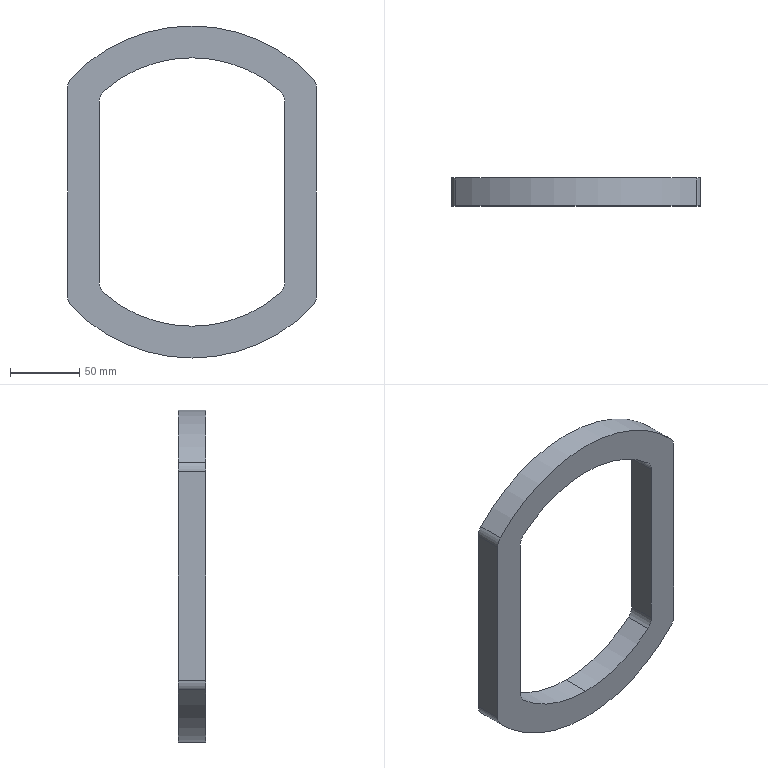Part | SolidWorks | features Extrusion 1, Fillet 1 | 1 solid | 20 faces | box 180 x 20 x 240 mm | volume 299340 mm3 | cylinder 14 | plane 6 | commonest cylinder face diameters 20 x8 194 x3 240 x3
STEP:
#1=CARTESIAN_POINT('',(63.552,20.,-73.282));
#2=VERTEX_POINT('',#1);
#3=CARTESIAN_POINT('',(0.,20.,-97.));
#4=VERTEX_POINT('',#3);
#5=CARTESIAN_POINT('',(0.,20.,0.));
#6=DIRECTION('',(0.,1.,0.));
#7=DIRECTION('',(0.,0.,1.));
#8=AXIS2_PLACEMENT_3D('',#5,#6,#7);
#9=CIRCLE('',#8,97.);
#10=EDGE_CURVE('',#2,#4,#9,.T.);
#11=ORIENTED_EDGE('',*,*,#10,.T.);
#12=CARTESIAN_POINT('',(0.,0.,-97.));
#13=VERTEX_POINT('',#12);
#14=CARTESIAN_POINT('',(0.,20.,-97.));
#15=DIRECTION('',(0.,-1.,0.));
#16=VECTOR('',#15,1000.);
#17=LINE('',#14,#16);
#18=EDGE_CURVE('',#4,#13,#17,.T.);
#19=ORIENTED_EDGE('',*,*,#18,.T.);
#20=CARTESIAN_POINT('',(63.552,0.,-73.282));
#21=VERTEX_POINT('',#20);
#22=CARTESIAN_POINT('',(0.,0.,0.));
#23=DIRECTION('',(0.,1.,0.));
#24=DIRECTION('',(0.,0.,1.));
#25=AXIS2_PLACEMENT_3D('',#22,#23,#24);
#26=CIRCLE('',#25,97.);
#27=EDGE_CURVE('',#21,#13,#26,.T.);
#28=ORIENTED_EDGE('',*,*,#27,.F.);
#29=CARTESIAN_POINT('',(63.552,20.,-73.282));
#30=DIRECTION('',(0.,1.,0.));
#31=VECTOR('',#30,1000.);
#32=LINE('',#29,#31);
#33=EDGE_CURVE('',#21,#2,#32,.T.);
#34=ORIENTED_EDGE('',*,*,#33,.T.);
#35=EDGE_LOOP('',(#11,#19,#28,#34));
#36=FACE_OUTER_BOUND('',#35,.T.);
#37=CARTESIAN_POINT('',(0.,20.,0.));
#38=DIRECTION('',(0.,-1.,0.));
#39=DIRECTION('',(0.,0.,-1.));
#40=AXIS2_PLACEMENT_3D('',#37,#38,#39);
#41=CYLINDRICAL_SURFACE('',#40,97.);
#42=ADVANCED_FACE('',(#36),#41,.F.);
#43=CARTESIAN_POINT('',(0.,20.,-120.));
#44=VERTEX_POINT('',#43);
#45=CARTESIAN_POINT('',(-87.273,20.,-82.362));
#46=VERTEX_POINT('',#45);
#47=CARTESIAN_POINT('',(0.,20.,0.));
#48=DIRECTION('',(0.,1.,0.));
#49=DIRECTION('',(0.,0.,1.));
#50=AXIS2_PLACEMENT_3D('',#47,#48,#49);
#51=CIRCLE('',#50,120.);
#52=EDGE_CURVE('',#44,#46,#51,.T.);
#53=ORIENTED_EDGE('',*,*,#52,.F.);
#54=CARTESIAN_POINT('',(0.,0.,-120.));
#55=VERTEX_POINT('',#54);
#56=CARTESIAN_POINT('',(0.,20.,-120.));
#57=DIRECTION('',(0.,-1.,0.));
#58=VECTOR('',#57,1000.);
#59=LINE('',#56,#58);
#60=EDGE_CURVE('',#44,#55,#59,.T.);
#61=ORIENTED_EDGE('',*,*,#60,.T.);
#62=CARTESIAN_POINT('',(-87.273,0.,-82.362));
#63=VERTEX_POINT('',#62);
#64=CARTESIAN_POINT('',(0.,0.,0.));
#65=DIRECTION('',(0.,1.,0.));
#66=DIRECTION('',(0.,0.,1.));
#67=AXIS2_PLACEMENT_3D('',#64,#65,#66);
#68=CIRCLE('',#67,120.);
#69=EDGE_CURVE('',#55,#63,#68,.T.);
#70=ORIENTED_EDGE('',*,*,#69,.T.);
#71=CARTESIAN_POINT('',(-87.273,20.,-82.362));
#72=DIRECTION('',(0.,-1.,0.));
#73=VECTOR('',#72,1000.);
#74=LINE('',#71,#73);
#75=EDGE_CURVE('',#46,#63,#74,.T.);
#76=ORIENTED_EDGE('',*,*,#75,.F.);
#77=EDGE_LOOP('',(#53,#61,#70,#76));
#78=FACE_OUTER_BOUND('',#77,.T.);
#79=CARTESIAN_POINT('',(0.,20.,0.));
#80=DIRECTION('',(0.,-1.,0.));
#81=DIRECTION('',(0.,0.,-1.));
#82=AXIS2_PLACEMENT_3D('',#79,#80,#81);
#83=CYLINDRICAL_SURFACE('',#82,120.);
#84=ADVANCED_FACE('',(#78),#83,.T.);
#85=CARTESIAN_POINT('',(90.,20.,-75.498));
#86=VERTEX_POINT('',#85);
#87=CARTESIAN_POINT('',(87.273,20.,-82.362));
#88=VERTEX_POINT('',#87);
#89=CARTESIAN_POINT('',(80.,20.,-75.498));
#90=DIRECTION('',(0.,1.,0.));
#91=DIRECTION('',(0.,0.,1.));
#92=AXIS2_PLACEMENT_3D('',#89,#90,#91);
#93=CIRCLE('',#92,10.);
#94=EDGE_CURVE('',#86,#88,#93,.T.);
#95=ORIENTED_EDGE('',*,*,#94,.T.);
#96=CARTESIAN_POINT('',(0.,20.,0.));
#97=DIRECTION('',(0.,1.,0.));
#98=DIRECTION('',(0.,0.,1.));
#99=AXIS2_PLACEMENT_3D('',#96,#97,#98);
#100=CIRCLE('',#99,120.);
#101=EDGE_CURVE('',#88,#44,#100,.T.);
#102=ORIENTED_EDGE('',*,*,#101,.T.);
#103=ORIENTED_EDGE('',*,*,#52,.T.);
#104=CARTESIAN_POINT('',(-90.,20.,-75.498));
#105=VERTEX_POINT('',#104);
#106=CARTESIAN_POINT('',(-80.,20.,-75.498));
#107=DIRECTION('',(0.,1.,0.));
#108=DIRECTION('',(0.,0.,1.));
#109=AXIS2_PLACEMENT_3D('',#106,#107,#108);
#110=CIRCLE('',#109,10.);
#111=EDGE_CURVE('',#46,#105,#110,.T.);
#112=ORIENTED_EDGE('',*,*,#111,.T.);
#113=CARTESIAN_POINT('',(-90.,20.,75.498));
#114=VERTEX_POINT('',#113);
#115=CARTESIAN_POINT('',(-90.,20.,-75.498));
#116=DIRECTION('',(0.,0.,1.));
#117=VECTOR('',#116,1000.);
#118=LINE('',#115,#117);
#119=EDGE_CURVE('',#105,#114,#118,.T.);
#120=ORIENTED_EDGE('',*,*,#119,.T.);
#121=CARTESIAN_POINT('',(-87.273,20.,82.362));
#122=VERTEX_POINT('',#121);
#123=CARTESIAN_POINT('',(-80.,20.,75.498));
#124=DIRECTION('',(0.,1.,0.));
#125=DIRECTION('',(0.,0.,1.));
#126=AXIS2_PLACEMENT_3D('',#123,#124,#125);
#127=CIRCLE('',#126,10.);
#128=EDGE_CURVE('',#114,#122,#127,.T.);
#129=ORIENTED_EDGE('',*,*,#128,.T.);
#130=CARTESIAN_POINT('',(87.273,20.,82.362));
#131=VERTEX_POINT('',#130);
#132=CARTESIAN_POINT('',(0.,20.,0.));
#133=DIRECTION('',(0.,1.,0.));
#134=DIRECTION('',(0.,0.,1.));
#135=AXIS2_PLACEMENT_3D('',#132,#133,#134);
#136=CIRCLE('',#135,120.);
#137=EDGE_CURVE('',#122,#131,#136,.T.);
#138=ORIENTED_EDGE('',*,*,#137,.T.);
#139=CARTESIAN_POINT('',(90.,20.,75.498));
#140=VERTEX_POINT('',#139);
#141=CARTESIAN_POINT('',(80.,20.,75.498));
#142=DIRECTION('',(0.,1.,0.));
#143=DIRECTION('',(0.,0.,1.));
#144=AXIS2_PLACEMENT_3D('',#141,#142,#143);
#145=CIRCLE('',#144,10.);
#146=EDGE_CURVE('',#131,#140,#145,.T.);
#147=ORIENTED_EDGE('',*,*,#146,.T.);
#148=CARTESIAN_POINT('',(90.,20.,75.498));
#149=DIRECTION('',(0.,0.,-1.));
#150=VECTOR('',#149,1000.);
#151=LINE('',#148,#150);
#152=EDGE_CURVE('',#140,#86,#151,.T.);
#153=ORIENTED_EDGE('',*,*,#152,.T.);
#154=EDGE_LOOP('',(#95,#102,#103,#112,#120,#129,#138,#147,#153));
#155=FACE_OUTER_BOUND('',#154,.T.);
#156=CARTESIAN_POINT('',(67.,20.,65.727));
#157=VERTEX_POINT('',#156);
#158=CARTESIAN_POINT('',(67.,20.,-65.727));
#159=VERTEX_POINT('',#158);
#160=CARTESIAN_POINT('',(67.,20.,70.143));
#161=DIRECTION('',(0.,0.,-1.));
#162=VECTOR('',#161,1000.);
#163=LINE('',#160,#162);
#164=EDGE_CURVE('',#157,#159,#163,.T.);
#165=ORIENTED_EDGE('',*,*,#164,.F.);
#166=CARTESIAN_POINT('',(63.552,20.,73.282));
#167=VERTEX_POINT('',#166);
#168=CARTESIAN_POINT('',(57.,20.,65.727));
#169=DIRECTION('',(0.,-1.,0.));
#170=DIRECTION('',(0.,0.,1.));
#171=AXIS2_PLACEMENT_3D('',#168,#169,#170);
#172=CIRCLE('',#171,10.);
#173=EDGE_CURVE('',#157,#167,#172,.T.);
#174=ORIENTED_EDGE('',*,*,#173,.T.);
#175=CARTESIAN_POINT('',(-63.552,20.,73.282));
#176=VERTEX_POINT('',#175);
#177=CARTESIAN_POINT('',(0.,20.,0.));
#178=DIRECTION('',(0.,1.,0.));
#179=DIRECTION('',(0.,0.,1.));
#180=AXIS2_PLACEMENT_3D('',#177,#178,#179);
#181=CIRCLE('',#180,97.);
#182=EDGE_CURVE('',#176,#167,#181,.T.);
#183=ORIENTED_EDGE('',*,*,#182,.F.);
#184=CARTESIAN_POINT('',(-67.,20.,65.727));
#185=VERTEX_POINT('',#184);
#186=CARTESIAN_POINT('',(-57.,20.,65.727));
#187=DIRECTION('',(0.,-1.,0.));
#188=DIRECTION('',(0.,0.,1.));
#189=AXIS2_PLACEMENT_3D('',#186,#187,#188);
#190=CIRCLE('',#189,10.);
#191=EDGE_CURVE('',#176,#185,#190,.T.);
#192=ORIENTED_EDGE('',*,*,#191,.T.);
#193=CARTESIAN_POINT('',(-67.,20.,-65.727));
#194=VERTEX_POINT('',#193);
#195=CARTESIAN_POINT('',(-67.,20.,-70.143));
#196=DIRECTION('',(0.,0.,1.));
#197=VECTOR('',#196,1000.);
#198=LINE('',#195,#197);
#199=EDGE_CURVE('',#194,#185,#198,.T.);
#200=ORIENTED_EDGE('',*,*,#199,.F.);
#201=CARTESIAN_POINT('',(-63.552,20.,-73.282));
#202=VERTEX_POINT('',#201);
#203=CARTESIAN_POINT('',(-57.,20.,-65.727));
#204=DIRECTION('',(0.,-1.,0.));
#205=DIRECTION('',(0.,0.,1.));
#206=AXIS2_PLACEMENT_3D('',#203,#204,#205);
#207=CIRCLE('',#206,10.);
#208=EDGE_CURVE('',#194,#202,#207,.T.);
#209=ORIENTED_EDGE('',*,*,#208,.T.);
#210=CARTESIAN_POINT('',(0.,20.,0.));
#211=DIRECTION('',(0.,1.,0.));
#212=DIRECTION('',(0.,0.,1.));
#213=AXIS2_PLACEMENT_3D('',#210,#211,#212);
#214=CIRCLE('',#213,97.);
#215=EDGE_CURVE('',#4,#202,#214,.T.);
#216=ORIENTED_EDGE('',*,*,#215,.F.);
#217=ORIENTED_EDGE('',*,*,#10,.F.);
#218=CARTESIAN_POINT('',(57.,20.,-65.727));
#219=DIRECTION('',(0.,-1.,0.));
#220=DIRECTION('',(0.,0.,1.));
#221=AXIS2_PLACEMENT_3D('',#218,#219,#220);
#222=CIRCLE('',#221,10.);
#223=EDGE_CURVE('',#2,#159,#222,.T.);
#224=ORIENTED_EDGE('',*,*,#223,.T.);
#225=EDGE_LOOP('',(#165,#174,#183,#192,#200,#209,#216,#217,#224));
#226=FACE_BOUND('',#225,.T.);
#227=CARTESIAN_POINT('',(80.,20.,-75.498));
#228=DIRECTION('',(0.,1.,0.));
#229=DIRECTION('',(0.,0.,1.));
#230=AXIS2_PLACEMENT_3D('',#227,#228,#229);
#231=PLANE('',#230);
#232=ADVANCED_FACE('',(#155,#226),#231,.T.);
#233=CARTESIAN_POINT('',(90.,0.,-75.498));
#234=VERTEX_POINT('',#233);
#235=CARTESIAN_POINT('',(87.273,0.,-82.362));
#236=VERTEX_POINT('',#235);
#237=CARTESIAN_POINT('',(80.,0.,-75.498));
#238=DIRECTION('',(0.,1.,0.));
#239=DIRECTION('',(0.,0.,1.));
#240=AXIS2_PLACEMENT_3D('',#237,#238,#239);
#241=CIRCLE('',#240,10.);
#242=EDGE_CURVE('',#234,#236,#241,.T.);
#243=ORIENTED_EDGE('',*,*,#242,.F.);
#244=CARTESIAN_POINT('',(90.,0.,75.498));
#245=VERTEX_POINT('',#244);
#246=CARTESIAN_POINT('',(90.,0.,75.498));
#247=DIRECTION('',(0.,0.,-1.));
#248=VECTOR('',#247,1000.);
#249=LINE('',#246,#248);
#250=EDGE_CURVE('',#245,#234,#249,.T.);
#251=ORIENTED_EDGE('',*,*,#250,.F.);
#252=CARTESIAN_POINT('',(87.273,0.,82.362));
#253=VERTEX_POINT('',#252);
#254=CARTESIAN_POINT('',(80.,0.,75.498));
#255=DIRECTION('',(0.,1.,0.));
#256=DIRECTION('',(0.,0.,1.));
#257=AXIS2_PLACEMENT_3D('',#254,#255,#256);
#258=CIRCLE('',#257,10.);
#259=EDGE_CURVE('',#253,#245,#258,.T.);
#260=ORIENTED_EDGE('',*,*,#259,.F.);
#261=CARTESIAN_POINT('',(-87.273,0.,82.362));
#262=VERTEX_POINT('',#261);
#263=CARTESIAN_POINT('',(0.,0.,0.));
#264=DIRECTION('',(0.,1.,0.));
#265=DIRECTION('',(0.,0.,1.));
#266=AXIS2_PLACEMENT_3D('',#263,#264,#265);
#267=CIRCLE('',#266,120.);
#268=EDGE_CURVE('',#262,#253,#267,.T.);
#269=ORIENTED_EDGE('',*,*,#268,.F.);
#270=CARTESIAN_POINT('',(-90.,0.,75.498));
#271=VERTEX_POINT('',#270);
#272=CARTESIAN_POINT('',(-80.,0.,75.498));
#273=DIRECTION('',(0.,1.,0.));
#274=DIRECTION('',(0.,0.,1.));
#275=AXIS2_PLACEMENT_3D('',#272,#273,#274);
#276=CIRCLE('',#275,10.);
#277=EDGE_CURVE('',#271,#262,#276,.T.);
#278=ORIENTED_EDGE('',*,*,#277,.F.);
#279=CARTESIAN_POINT('',(-90.,0.,-75.498));
#280=VERTEX_POINT('',#279);
#281=CARTESIAN_POINT('',(-90.,0.,-75.498));
#282=DIRECTION('',(0.,0.,1.));
#283=VECTOR('',#282,1000.);
#284=LINE('',#281,#283);
#285=EDGE_CURVE('',#280,#271,#284,.T.);
#286=ORIENTED_EDGE('',*,*,#285,.F.);
#287=CARTESIAN_POINT('',(-80.,0.,-75.498));
#288=DIRECTION('',(0.,1.,0.));
#289=DIRECTION('',(0.,0.,1.));
#290=AXIS2_PLACEMENT_3D('',#287,#288,#289);
#291=CIRCLE('',#290,10.);
#292=EDGE_CURVE('',#63,#280,#291,.T.);
#293=ORIENTED_EDGE('',*,*,#292,.F.);
#294=ORIENTED_EDGE('',*,*,#69,.F.);
#295=CARTESIAN_POINT('',(0.,0.,0.));
#296=DIRECTION('',(0.,1.,0.));
#297=DIRECTION('',(0.,0.,1.));
#298=AXIS2_PLACEMENT_3D('',#295,#296,#297);
#299=CIRCLE('',#298,120.);
#300=EDGE_CURVE('',#236,#55,#299,.T.);
#301=ORIENTED_EDGE('',*,*,#300,.F.);
#302=EDGE_LOOP('',(#243,#251,#260,#269,#278,#286,#293,#294,#301));
#303=FACE_OUTER_BOUND('',#302,.T.);
#304=CARTESIAN_POINT('',(-67.,0.,-65.727));
#305=VERTEX_POINT('',#304);
#306=CARTESIAN_POINT('',(-67.,0.,65.727));
#307=VERTEX_POINT('',#306);
#308=CARTESIAN_POINT('',(-67.,0.,-70.143));
#309=DIRECTION('',(0.,0.,1.));
#310=VECTOR('',#309,1000.);
#311=LINE('',#308,#310);
#312=EDGE_CURVE('',#305,#307,#311,.T.);
#313=ORIENTED_EDGE('',*,*,#312,.T.);
#314=CARTESIAN_POINT('',(-63.552,0.,73.282));
#315=VERTEX_POINT('',#314);
#316=CARTESIAN_POINT('',(-57.,0.,65.727));
#317=DIRECTION('',(0.,1.,0.));
#318=DIRECTION('',(0.,0.,1.));
#319=AXIS2_PLACEMENT_3D('',#316,#317,#318);
#320=CIRCLE('',#319,10.);
#321=EDGE_CURVE('',#307,#315,#320,.T.);
#322=ORIENTED_EDGE('',*,*,#321,.T.);
#323=CARTESIAN_POINT('',(63.552,0.,73.282));
#324=VERTEX_POINT('',#323);
#325=CARTESIAN_POINT('',(0.,0.,0.));
#326=DIRECTION('',(0.,1.,0.));
#327=DIRECTION('',(0.,0.,1.));
#328=AXIS2_PLACEMENT_3D('',#325,#326,#327);
#329=CIRCLE('',#328,97.);
#330=EDGE_CURVE('',#315,#324,#329,.T.);
#331=ORIENTED_EDGE('',*,*,#330,.T.);
#332=CARTESIAN_POINT('',(67.,0.,65.727));
#333=VERTEX_POINT('',#332);
#334=CARTESIAN_POINT('',(57.,0.,65.727));
#335=DIRECTION('',(0.,1.,0.));
#336=DIRECTION('',(0.,0.,1.));
#337=AXIS2_PLACEMENT_3D('',#334,#335,#336);
#338=CIRCLE('',#337,10.);
#339=EDGE_CURVE('',#324,#333,#338,.T.);
#340=ORIENTED_EDGE('',*,*,#339,.T.);
#341=CARTESIAN_POINT('',(67.,0.,-65.727));
#342=VERTEX_POINT('',#341);
#343=CARTESIAN_POINT('',(67.,0.,70.143));
#344=DIRECTION('',(0.,0.,-1.));
#345=VECTOR('',#344,1000.);
#346=LINE('',#343,#345);
#347=EDGE_CURVE('',#333,#342,#346,.T.);
#348=ORIENTED_EDGE('',*,*,#347,.T.);
#349=CARTESIAN_POINT('',(57.,0.,-65.727));
#350=DIRECTION('',(0.,1.,0.));
#351=DIRECTION('',(0.,0.,1.));
#352=AXIS2_PLACEMENT_3D('',#349,#350,#351);
#353=CIRCLE('',#352,10.);
#354=EDGE_CURVE('',#342,#21,#353,.T.);
#355=ORIENTED_EDGE('',*,*,#354,.T.);
#356=ORIENTED_EDGE('',*,*,#27,.T.);
#357=CARTESIAN_POINT('',(-63.552,0.,-73.282));
#358=VERTEX_POINT('',#357);
#359=CARTESIAN_POINT('',(0.,0.,0.));
#360=DIRECTION('',(0.,1.,0.));
#361=DIRECTION('',(0.,0.,1.));
#362=AXIS2_PLACEMENT_3D('',#359,#360,#361);
#363=CIRCLE('',#362,97.);
#364=EDGE_CURVE('',#13,#358,#363,.T.);
#365=ORIENTED_EDGE('',*,*,#364,.T.);
#366=CARTESIAN_POINT('',(-57.,0.,-65.727));
#367=DIRECTION('',(0.,1.,0.));
#368=DIRECTION('',(0.,0.,1.));
#369=AXIS2_PLACEMENT_3D('',#366,#367,#368);
#370=CIRCLE('',#369,10.);
#371=EDGE_CURVE('',#358,#305,#370,.T.);
#372=ORIENTED_EDGE('',*,*,#371,.T.);
#373=EDGE_LOOP('',(#313,#322,#331,#340,#348,#355,#356,#365,#372));
#374=FACE_BOUND('',#373,.T.);
#375=CARTESIAN_POINT('',(80.,0.,-75.498));
#376=DIRECTION('',(0.,1.,0.));
#377=DIRECTION('',(0.,0.,1.));
#378=AXIS2_PLACEMENT_3D('',#375,#376,#377);
#379=PLANE('',#378);
#380=ADVANCED_FACE('',(#303,#374),#379,.F.);
#381=ORIENTED_EDGE('',*,*,#242,.T.);
#382=CARTESIAN_POINT('',(87.273,20.,-82.362));
#383=DIRECTION('',(0.,-1.,0.));
#384=VECTOR('',#383,1000.);
#385=LINE('',#382,#384);
#386=EDGE_CURVE('',#88,#236,#385,.T.);
#387=ORIENTED_EDGE('',*,*,#386,.F.);
#388=ORIENTED_EDGE('',*,*,#94,.F.);
#389=CARTESIAN_POINT('',(90.,20.,-75.498));
#390=DIRECTION('',(0.,-1.,0.));
#391=VECTOR('',#390,1000.);
#392=LINE('',#389,#391);
#393=EDGE_CURVE('',#86,#234,#392,.T.);
#394=ORIENTED_EDGE('',*,*,#393,.T.);
#395=EDGE_LOOP('',(#381,#387,#388,#394));
#396=FACE_OUTER_BOUND('',#395,.T.);
#397=CARTESIAN_POINT('',(80.,20.,-75.498));
#398=DIRECTION('',(0.,-1.,0.));
#399=DIRECTION('',(0.,0.,-1.));
#400=AXIS2_PLACEMENT_3D('',#397,#398,#399);
#401=CYLINDRICAL_SURFACE('',#400,10.);
#402=ADVANCED_FACE('',(#396),#401,.T.);
#403=ORIENTED_EDGE('',*,*,#60,.F.);
#404=ORIENTED_EDGE('',*,*,#101,.F.);
#405=ORIENTED_EDGE('',*,*,#386,.T.);
#406=ORIENTED_EDGE('',*,*,#300,.T.);
#407=EDGE_LOOP('',(#403,#404,#405,#406));
#408=FACE_OUTER_BOUND('',#407,.T.);
#409=CARTESIAN_POINT('',(0.,20.,0.));
#410=DIRECTION('',(0.,-1.,0.));
#411=DIRECTION('',(0.,0.,-1.));
#412=AXIS2_PLACEMENT_3D('',#409,#410,#411);
#413=CYLINDRICAL_SURFACE('',#412,120.);
#414=ADVANCED_FACE('',(#408),#413,.T.);
#415=ORIENTED_EDGE('',*,*,#292,.T.);
#416=CARTESIAN_POINT('',(-90.,20.,-75.498));
#417=DIRECTION('',(0.,-1.,0.));
#418=VECTOR('',#417,1000.);
#419=LINE('',#416,#418);
#420=EDGE_CURVE('',#105,#280,#419,.T.);
#421=ORIENTED_EDGE('',*,*,#420,.F.);
#422=ORIENTED_EDGE('',*,*,#111,.F.);
#423=ORIENTED_EDGE('',*,*,#75,.T.);
#424=EDGE_LOOP('',(#415,#421,#422,#423));
#425=FACE_OUTER_BOUND('',#424,.T.);
#426=CARTESIAN_POINT('',(-80.,20.,-75.498));
#427=DIRECTION('',(0.,-1.,0.));
#428=DIRECTION('',(0.,0.,-1.));
#429=AXIS2_PLACEMENT_3D('',#426,#427,#428);
#430=CYLINDRICAL_SURFACE('',#429,10.);
#431=ADVANCED_FACE('',(#425),#430,.T.);
#432=ORIENTED_EDGE('',*,*,#285,.T.);
#433=CARTESIAN_POINT('',(-90.,20.,75.498));
#434=DIRECTION('',(0.,-1.,0.));
#435=VECTOR('',#434,1000.);
#436=LINE('',#433,#435);
#437=EDGE_CURVE('',#114,#271,#436,.T.);
#438=ORIENTED_EDGE('',*,*,#437,.F.);
#439=ORIENTED_EDGE('',*,*,#119,.F.);
#440=ORIENTED_EDGE('',*,*,#420,.T.);
#441=EDGE_LOOP('',(#432,#438,#439,#440));
#442=FACE_OUTER_BOUND('',#441,.T.);
#443=CARTESIAN_POINT('',(-90.,20.,-75.498));
#444=DIRECTION('',(1.,0.,0.));
#445=DIRECTION('',(0.,0.,-1.));
#446=AXIS2_PLACEMENT_3D('',#443,#444,#445);
#447=PLANE('',#446);
#448=ADVANCED_FACE('',(#442),#447,.F.);
#449=ORIENTED_EDGE('',*,*,#277,.T.);
#450=CARTESIAN_POINT('',(-87.273,20.,82.362));
#451=DIRECTION('',(0.,-1.,0.));
#452=VECTOR('',#451,1000.);
#453=LINE('',#450,#452);
#454=EDGE_CURVE('',#122,#262,#453,.T.);
#455=ORIENTED_EDGE('',*,*,#454,.F.);
#456=ORIENTED_EDGE('',*,*,#128,.F.);
#457=ORIENTED_EDGE('',*,*,#437,.T.);
#458=EDGE_LOOP('',(#449,#455,#456,#457));
#459=FACE_OUTER_BOUND('',#458,.T.);
#460=CARTESIAN_POINT('',(-80.,20.,75.498));
#461=DIRECTION('',(0.,-1.,0.));
#462=DIRECTION('',(0.,0.,-1.));
#463=AXIS2_PLACEMENT_3D('',#460,#461,#462);
#464=CYLINDRICAL_SURFACE('',#463,10.);
#465=ADVANCED_FACE('',(#459),#464,.T.);
#466=ORIENTED_EDGE('',*,*,#268,.T.);
#467=CARTESIAN_POINT('',(87.273,20.,82.362));
#468=DIRECTION('',(0.,-1.,0.));
#469=VECTOR('',#468,1000.);
#470=LINE('',#467,#469);
#471=EDGE_CURVE('',#131,#253,#470,.T.);
#472=ORIENTED_EDGE('',*,*,#471,.F.);
#473=ORIENTED_EDGE('',*,*,#137,.F.);
#474=ORIENTED_EDGE('',*,*,#454,.T.);
#475=EDGE_LOOP('',(#466,#472,#473,#474));
#476=FACE_OUTER_BOUND('',#475,.T.);
#477=CARTESIAN_POINT('',(0.,20.,0.));
#478=DIRECTION('',(0.,-1.,0.));
#479=DIRECTION('',(0.,0.,-1.));
#480=AXIS2_PLACEMENT_3D('',#477,#478,#479);
#481=CYLINDRICAL_SURFACE('',#480,120.);
#482=ADVANCED_FACE('',(#476),#481,.T.);
#483=ORIENTED_EDGE('',*,*,#259,.T.);
#484=CARTESIAN_POINT('',(90.,20.,75.498));
#485=DIRECTION('',(0.,-1.,0.));
#486=VECTOR('',#485,1000.);
#487=LINE('',#484,#486);
#488=EDGE_CURVE('',#140,#245,#487,.T.);
#489=ORIENTED_EDGE('',*,*,#488,.F.);
#490=ORIENTED_EDGE('',*,*,#146,.F.);
#491=ORIENTED_EDGE('',*,*,#471,.T.);
#492=EDGE_LOOP('',(#483,#489,#490,#491));
#493=FACE_OUTER_BOUND('',#492,.T.);
#494=CARTESIAN_POINT('',(80.,20.,75.498));
#495=DIRECTION('',(0.,-1.,0.));
#496=DIRECTION('',(0.,0.,-1.));
#497=AXIS2_PLACEMENT_3D('',#494,#495,#496);
#498=CYLINDRICAL_SURFACE('',#497,10.);
#499=ADVANCED_FACE('',(#493),#498,.T.);
#500=ORIENTED_EDGE('',*,*,#250,.T.);
#501=ORIENTED_EDGE('',*,*,#393,.F.);
#502=ORIENTED_EDGE('',*,*,#152,.F.);
#503=ORIENTED_EDGE('',*,*,#488,.T.);
#504=EDGE_LOOP('',(#500,#501,#502,#503));
#505=FACE_OUTER_BOUND('',#504,.T.);
#506=CARTESIAN_POINT('',(90.,20.,75.498));
#507=DIRECTION('',(-1.,0.,0.));
#508=DIRECTION('',(0.,0.,1.));
#509=AXIS2_PLACEMENT_3D('',#506,#507,#508);
#510=PLANE('',#509);
#511=ADVANCED_FACE('',(#505),#510,.F.);
#512=ORIENTED_EDGE('',*,*,#330,.F.);
#513=CARTESIAN_POINT('',(-63.552,20.,73.282));
#514=DIRECTION('',(0.,1.,0.));
#515=VECTOR('',#514,1000.);
#516=LINE('',#513,#515);
#517=EDGE_CURVE('',#315,#176,#516,.T.);
#518=ORIENTED_EDGE('',*,*,#517,.T.);
#519=ORIENTED_EDGE('',*,*,#182,.T.);
#520=CARTESIAN_POINT('',(63.552,20.,73.282));
#521=DIRECTION('',(0.,-1.,0.));
#522=VECTOR('',#521,1000.);
#523=LINE('',#520,#522);
#524=EDGE_CURVE('',#167,#324,#523,.T.);
#525=ORIENTED_EDGE('',*,*,#524,.T.);
#526=EDGE_LOOP('',(#512,#518,#519,#525));
#527=FACE_OUTER_BOUND('',#526,.T.);
#528=CARTESIAN_POINT('',(0.,20.,0.));
#529=DIRECTION('',(0.,-1.,0.));
#530=DIRECTION('',(0.,0.,-1.));
#531=AXIS2_PLACEMENT_3D('',#528,#529,#530);
#532=CYLINDRICAL_SURFACE('',#531,97.);
#533=ADVANCED_FACE('',(#527),#532,.F.);
#534=ORIENTED_EDGE('',*,*,#164,.T.);
#535=CARTESIAN_POINT('',(67.,0.,-65.727));
#536=DIRECTION('',(0.,-1.,0.));
#537=VECTOR('',#536,1000.);
#538=LINE('',#535,#537);
#539=EDGE_CURVE('',#159,#342,#538,.T.);
#540=ORIENTED_EDGE('',*,*,#539,.T.);
#541=ORIENTED_EDGE('',*,*,#347,.F.);
#542=CARTESIAN_POINT('',(67.,20.,65.727));
#543=DIRECTION('',(0.,1.,0.));
#544=VECTOR('',#543,1000.);
#545=LINE('',#542,#544);
#546=EDGE_CURVE('',#333,#157,#545,.T.);
#547=ORIENTED_EDGE('',*,*,#546,.T.);
#548=EDGE_LOOP('',(#534,#540,#541,#547));
#549=FACE_OUTER_BOUND('',#548,.T.);
#550=CARTESIAN_POINT('',(67.,20.,70.143));
#551=DIRECTION('',(-1.,0.,0.));
#552=DIRECTION('',(0.,0.,1.));
#553=AXIS2_PLACEMENT_3D('',#550,#551,#552);
#554=PLANE('',#553);
#555=ADVANCED_FACE('',(#549),#554,.T.);
#556=ORIENTED_EDGE('',*,*,#18,.F.);
#557=ORIENTED_EDGE('',*,*,#215,.T.);
#558=CARTESIAN_POINT('',(-63.552,20.,-73.282));
#559=DIRECTION('',(0.,-1.,0.));
#560=VECTOR('',#559,1000.);
#561=LINE('',#558,#560);
#562=EDGE_CURVE('',#202,#358,#561,.T.);
#563=ORIENTED_EDGE('',*,*,#562,.T.);
#564=ORIENTED_EDGE('',*,*,#364,.F.);
#565=EDGE_LOOP('',(#556,#557,#563,#564));
#566=FACE_OUTER_BOUND('',#565,.T.);
#567=CARTESIAN_POINT('',(0.,20.,0.));
#568=DIRECTION('',(0.,-1.,0.));
#569=DIRECTION('',(0.,0.,-1.));
#570=AXIS2_PLACEMENT_3D('',#567,#568,#569);
#571=CYLINDRICAL_SURFACE('',#570,97.);
#572=ADVANCED_FACE('',(#566),#571,.F.);
#573=ORIENTED_EDGE('',*,*,#199,.T.);
#574=CARTESIAN_POINT('',(-67.,0.,65.727));
#575=DIRECTION('',(0.,-1.,0.));
#576=VECTOR('',#575,1000.);
#577=LINE('',#574,#576);
#578=EDGE_CURVE('',#185,#307,#577,.T.);
#579=ORIENTED_EDGE('',*,*,#578,.T.);
#580=ORIENTED_EDGE('',*,*,#312,.F.);
#581=CARTESIAN_POINT('',(-67.,20.,-65.727));
#582=DIRECTION('',(0.,1.,0.));
#583=VECTOR('',#582,1000.);
#584=LINE('',#581,#583);
#585=EDGE_CURVE('',#305,#194,#584,.T.);
#586=ORIENTED_EDGE('',*,*,#585,.T.);
#587=EDGE_LOOP('',(#573,#579,#580,#586));
#588=FACE_OUTER_BOUND('',#587,.T.);
#589=CARTESIAN_POINT('',(-67.,20.,-70.143));
#590=DIRECTION('',(1.,0.,0.));
#591=DIRECTION('',(0.,0.,-1.));
#592=AXIS2_PLACEMENT_3D('',#589,#590,#591);
#593=PLANE('',#592);
#594=ADVANCED_FACE('',(#588),#593,.T.);
#595=ORIENTED_EDGE('',*,*,#223,.F.);
#596=ORIENTED_EDGE('',*,*,#33,.F.);
#597=ORIENTED_EDGE('',*,*,#354,.F.);
#598=ORIENTED_EDGE('',*,*,#539,.F.);
#599=EDGE_LOOP('',(#595,#596,#597,#598));
#600=FACE_OUTER_BOUND('',#599,.T.);
#601=CARTESIAN_POINT('',(57.,20.,-65.727));
#602=DIRECTION('',(0.,-1.,0.));
#603=DIRECTION('',(0.,0.,-1.));
#604=AXIS2_PLACEMENT_3D('',#601,#602,#603);
#605=CYLINDRICAL_SURFACE('',#604,10.);
#606=ADVANCED_FACE('',(#600),#605,.F.);
#607=ORIENTED_EDGE('',*,*,#191,.F.);
#608=ORIENTED_EDGE('',*,*,#517,.F.);
#609=ORIENTED_EDGE('',*,*,#321,.F.);
#610=ORIENTED_EDGE('',*,*,#578,.F.);
#611=EDGE_LOOP('',(#607,#608,#609,#610));
#612=FACE_OUTER_BOUND('',#611,.T.);
#613=CARTESIAN_POINT('',(-57.,20.,65.727));
#614=DIRECTION('',(0.,-1.,0.));
#615=DIRECTION('',(0.,0.,-1.));
#616=AXIS2_PLACEMENT_3D('',#613,#614,#615);
#617=CYLINDRICAL_SURFACE('',#616,10.);
#618=ADVANCED_FACE('',(#612),#617,.F.);
#619=ORIENTED_EDGE('',*,*,#173,.F.);
#620=ORIENTED_EDGE('',*,*,#546,.F.);
#621=ORIENTED_EDGE('',*,*,#339,.F.);
#622=ORIENTED_EDGE('',*,*,#524,.F.);
#623=EDGE_LOOP('',(#619,#620,#621,#622));
#624=FACE_OUTER_BOUND('',#623,.T.);
#625=CARTESIAN_POINT('',(57.,20.,65.727));
#626=DIRECTION('',(0.,-1.,0.));
#627=DIRECTION('',(0.,0.,-1.));
#628=AXIS2_PLACEMENT_3D('',#625,#626,#627);
#629=CYLINDRICAL_SURFACE('',#628,10.);
#630=ADVANCED_FACE('',(#624),#629,.F.);
#631=ORIENTED_EDGE('',*,*,#208,.F.);
#632=ORIENTED_EDGE('',*,*,#585,.F.);
#633=ORIENTED_EDGE('',*,*,#371,.F.);
#634=ORIENTED_EDGE('',*,*,#562,.F.);
#635=EDGE_LOOP('',(#631,#632,#633,#634));
#636=FACE_OUTER_BOUND('',#635,.T.);
#637=CARTESIAN_POINT('',(-57.,20.,-65.727));
#638=DIRECTION('',(0.,-1.,0.));
#639=DIRECTION('',(0.,0.,-1.));
#640=AXIS2_PLACEMENT_3D('',#637,#638,#639);
#641=CYLINDRICAL_SURFACE('',#640,10.);
#642=ADVANCED_FACE('',(#636),#641,.F.);
#643=CLOSED_SHELL('',(#42,#84,#232,#380,#402,#414,#431,#448,#465,#482,#499,#511,#533,#555,#572,#594,#606,#618,#630,#642));
#644=MANIFOLD_SOLID_BREP('',#643);
#645=CARTESIAN_POINT('',(0.,0.,0.));
#646=DIRECTION('',(0.,0.,1.));
#647=DIRECTION('',(1.,0.,0.));
#648=AXIS2_PLACEMENT_3D('',#645,#646,#647);
#649=(LENGTH_UNIT()NAMED_UNIT(*)SI_UNIT(.MILLI.,.METRE.));
#650=UNCERTAINTY_MEASURE_WITH_UNIT(LENGTH_MEASURE(0.00001),#649,'','');
#651=(NAMED_UNIT(*)PLANE_ANGLE_UNIT()SI_UNIT($,.RADIAN.));
#652=(NAMED_UNIT(*)SI_UNIT($,.STERADIAN.)SOLID_ANGLE_UNIT());
#653=(GEOMETRIC_REPRESENTATION_CONTEXT(3)GLOBAL_UNCERTAINTY_ASSIGNED_CONTEXT((#650))GLOBAL_UNIT_ASSIGNED_CONTEXT((#649,#651,#652))REPRESENTATION_CONTEXT('',''));
#654=ADVANCED_BREP_SHAPE_REPRESENTATION('',(#644,#648),#653);